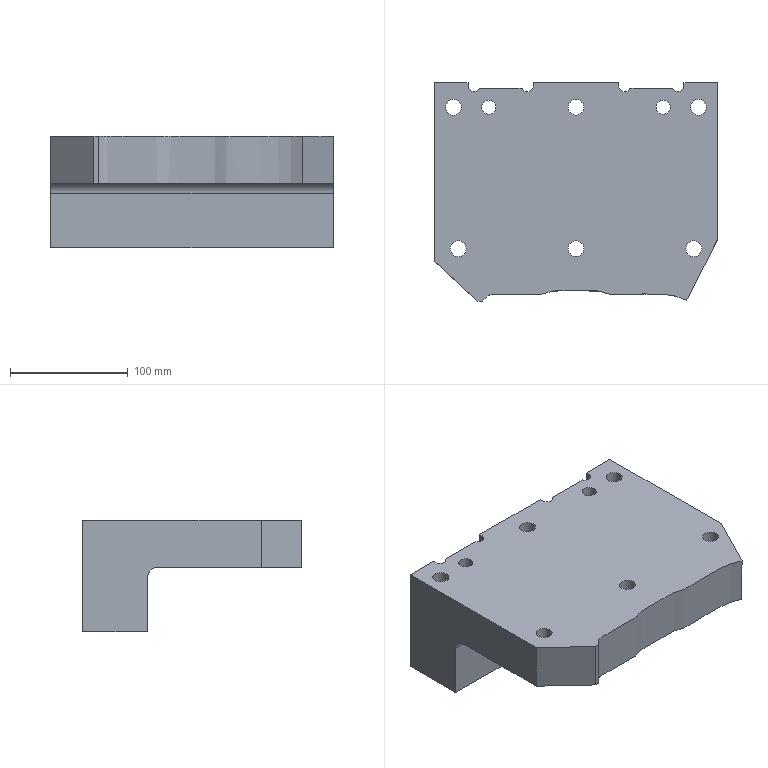Part | NX | features solid 2 | 1 solid | 64 faces | box 240 x 185.752 x 95 mm | volume 2207945 mm3 | cylinder 27 | plane 25 | cone 10 | spline 2 | commonest cylinder face diameters 13.507 x6 20.008 x6 10 x4 10.3 x4 10.506 x2 12 x2